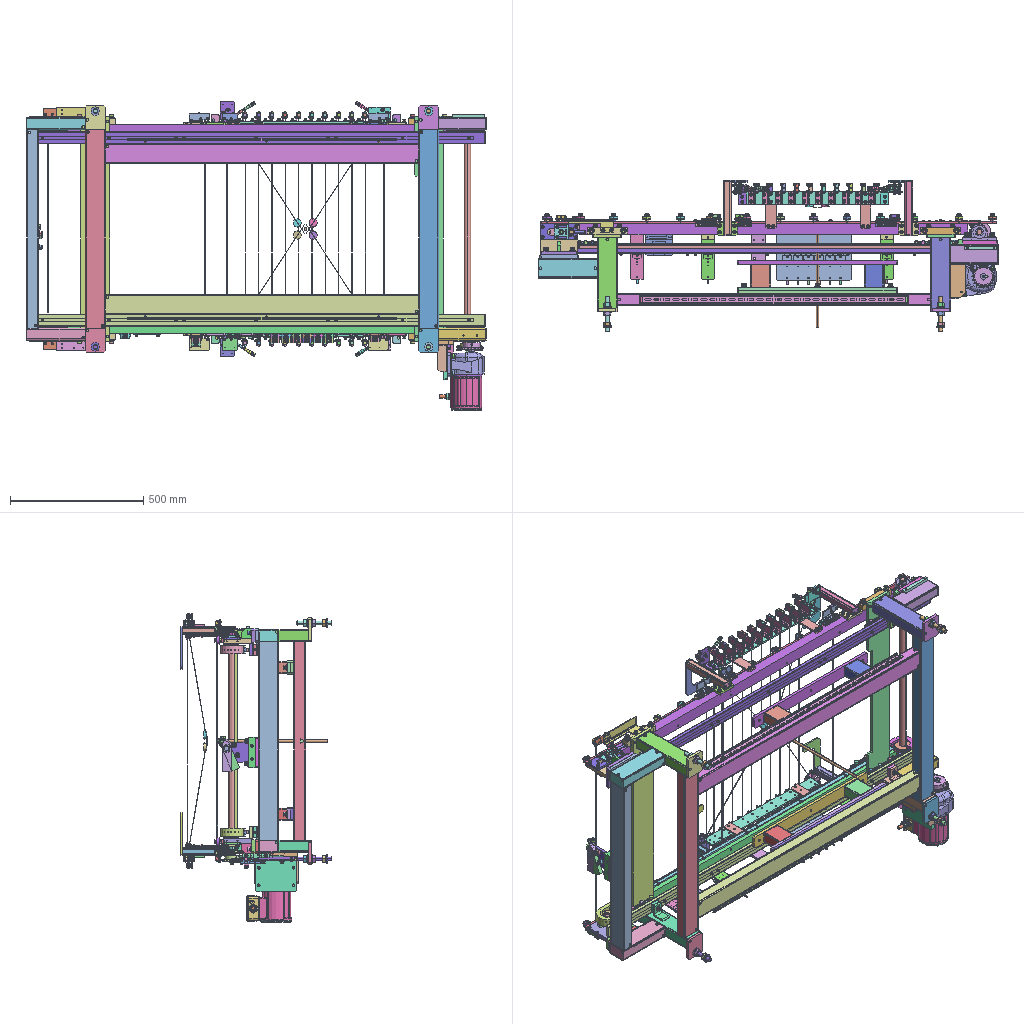Assembly | STEP file | 1685 different items | 2041 placed | box 1725 x 566 x 1158 mm
Parts list (item | name | quantity | parent item | size | volume), first 292 of 1685 items:
1 | 30B-162015T | x1 | in J306-EBZ05-01-40 | 15 x 20 x 20 mm | 1686 mm3
2 | AJSTS8-45 | x1 | in [1 unit purchased part] | 78 x 15.011 x 13 mm | 5597 mm3
3 | BB62-M10-25L | x1 | in J013-EBZ05-13-06 | 16 x 35 x 16 mm | 3564 mm3
4 | BB62-M10-25L-1 | x1 | in J013-EBZ05-13-06 | 16 x 35 x 16 mm | 3564 mm3
5 | BB62-M10-25L-10 | x1 | in J013-EBZ05-13-06 | 16 x 35 x 16 mm | 3564 mm3
6 | BB62-M10-25L-11 | x1 | in J013-EBZ05-13-06 | 16 x 35 x 16 mm | 3564 mm3
7 | BB62-M10-25L-12 | x1 | in J013-EBZ05-13-06 | 16 x 35 x 16 mm | 3564 mm3
8 | BB62-M10-25L-13 | x1 | in J013-EBZ05-13-06 | 16 x 35 x 16 mm | 3564 mm3
9 | BB62-M10-25L-14 | x1 | in J013-EBZ05-12-06 | 16 x 35 x 16 mm | 3564 mm3
10 | BB62-M10-25L-15 | x1 | in J013-EBZ05-12-06 | 16 x 35 x 16 mm | 3564 mm3
11 | BB62-M10-25L-16 | x1 | in J013-EBZ05-12-06 | 16 x 35 x 16 mm | 3564 mm3
12 | BB62-M10-25L-17 | x1 | in J013-EBZ05-12-06 | 16 x 35 x 16 mm | 3564 mm3
13 | BB62-M10-25L-18 | x1 | in J013-EBZ05-12-06 | 16 x 35 x 16 mm | 3564 mm3
14 | BB62-M10-25L-19 | x1 | in J013-EBZ05-12-06 | 16 x 35 x 16 mm | 3564 mm3
15 | BB62-M10-25L-2 | x1 | in J013-EBZ05-13-06 | 16 x 35 x 16 mm | 3564 mm3
16 | BB62-M10-25L-20 | x1 | in J013-EBZ05-12-06 | 16 x 35 x 16 mm | 3564 mm3
17 | BB62-M10-25L-21 | x1 | in J013-EBZ05-12-06 | 16 x 35 x 16 mm | 3564 mm3
18 | BB62-M10-25L-22 | x1 | in J013-EBZ05-12-06 | 16 x 35 x 16 mm | 3564 mm3
19 | BB62-M10-25L-23 | x1 | in J013-EBZ05-12-06 | 16 x 35 x 16 mm | 3564 mm3
20 | BB62-M10-25L-24 | x1 | in J013-EBZ05-12-06 | 16 x 35 x 16 mm | 3564 mm3
21 | BB62-M10-25L-25 | x1 | in J013-EBZ05-12-06 | 16 x 35 x 16 mm | 3564 mm3
22 | BB62-M10-25L-26 | x1 | in J013-EBZ05-12-06 | 16 x 35 x 16 mm | 3564 mm3
23 | BB62-M10-25L-27 | x1 | in J013-EBZ05-12-06 | 16 x 35 x 16 mm | 3564 mm3
24 | BB62-M10-25L-3 | x1 | in J013-EBZ05-13-06 | 16 x 35 x 16 mm | 3564 mm3
25 | BB62-M10-25L-4 | x1 | in J013-EBZ05-13-06 | 16 x 35 x 16 mm | 3564 mm3
26 | BB62-M10-25L-5 | x1 | in J013-EBZ05-13-06 | 16 x 35 x 16 mm | 3564 mm3
27 | BB62-M10-25L-6 | x1 | in J013-EBZ05-13-06 | 16 x 35 x 16 mm | 3564 mm3
28 | BB62-M10-25L-7 | x1 | in J013-EBZ05-13-06 | 16 x 35 x 16 mm | 3564 mm3
29 | BB62-M10-25L-8 | x1 | in J013-EBZ05-13-06 | 16 x 35 x 16 mm | 3564 mm3
30 | BB62-M10-25L-9 | x1 | in J013-EBZ05-13-06 | 16 x 35 x 16 mm | 3564 mm3
31 | BB62-M10-30L | x1 | in [1 unit purchased part] | 16 x 40 x 16 mm | 3957 mm3
32 | BB62-M10-30L-1 | x1 | in [1 unit purchased part] | 16 x 40 x 16 mm | 3957 mm3
33 | BB62-M10-30L-10 | x1 | - | 16 x 40 x 16 mm | 3957 mm3
34 | BB62-M10-30L-11 | x1 | - | 16 x 40 x 16 mm | 3957 mm3
35 | BB62-M10-30L-2 | x1 | in [1 unit purchased part] | 16 x 40 x 16 mm | 3957 mm3
36 | BB62-M10-30L-3 | x1 | in [1 unit purchased part] | 16 x 40 x 16 mm | 3957 mm3
37 | BB62-M10-30L-4 | x1 | - | 16 x 40 x 16 mm | 3957 mm3
38 | BB62-M10-30L-5 | x1 | - | 16 x 40 x 16 mm | 3957 mm3
39 | BB62-M10-30L-6 | x1 | - | 16 x 40 x 16 mm | 3957 mm3
40 | BB62-M10-30L-7 | x1 | - | 16 x 40 x 16 mm | 3957 mm3
41 | BB62-M10-30L-8 | x1 | - | 16 x 40 x 16 mm | 3957 mm3
42 | BB62-M10-30L-9 | x1 | - | 16 x 40 x 16 mm | 3957 mm3
43 | BB62-M10-35L | x1 | - | 16 x 45 x 16 mm | 4350 mm3
44 | BB62-M10-35L-1 | x1 | - | 16 x 45 x 16 mm | 4350 mm3
45 | BB62-M10-35L-2 | x1 | - | 16 x 45 x 16 mm | 4350 mm3
46 | BB62-M10-35L-3 | x1 | - | 16 x 45 x 16 mm | 4350 mm3
47 | BB62-M10-40L | x2 | in J013-EBZ05-14-06 | 16 x 50 x 16 mm | 4742 mm3
48 | BB62-M10-40L-1 | x2 | in J013-EBZ05-14-06 | 16 x 50 x 16 mm | 4742 mm3
49 | BB62-M10-40L-2 | x2 | in J013-EBZ05-28-06 | 16 x 50 x 16 mm | 4742 mm3
50 | BB62-M10-40L-3 | x2 | in J013-EBZ05-28-06 | 16 x 50 x 16 mm | 4742 mm3
51 | BB62-M10-40L-4 | x1 | - | 16 x 50 x 16 mm | 4742 mm3
52 | BB62-M10-40L-5 | x1 | - | 16 x 50 x 16 mm | 4742 mm3
53 | BB62-M10-45L | x2 | in J013-EBZ05-14-06 | 16 x 55 x 16 mm | 5135 mm3
54 | BB62-M10-45L-1 | x2 | in J013-EBZ05-14-06 | 16 x 55 x 16 mm | 5135 mm3
55 | BB62-M10-45L-2 | x2 | in J013-EBZ05-28-06 | 16 x 55 x 16 mm | 5135 mm3
56 | BB62-M10-45L-3 | x2 | in J013-EBZ05-28-06 | 16 x 55 x 16 mm | 5135 mm3
57 | BB62-M12-30L | x2 | in J011-EBZ05-05-00 | 18 x 42 x 18 mm | 5695 mm3
58 | BB62-M12-30L-1 | x2 | in J011-EBZ05-05-00 | 18 x 42 x 18 mm | 5695 mm3
59 | BB62-M3-10L | x1 | - | 5.5 x 13 x 5.5 mm | 130.673 mm3
60 | BB62-M3-10L-1 | x1 | - | 5.5 x 13 x 5.5 mm | 130.673 mm3
61 | BB62-M3-10L-10 | x10 | in J014-EBZ05-07-06 | 5.5 x 13 x 5.5 mm | 130.673 mm3
62 | BB62-M3-10L-11 | x10 | in J014-EBZ05-07-06 | 5.5 x 13 x 5.5 mm | 130.673 mm3
63 | BB62-M3-10L-12 | x1 | in J014-EBZ05-13-06 | 5.5 x 13 x 5.5 mm | 130.673 mm3
64 | BB62-M3-10L-13 | x1 | in J014-EBZ05-13-06 | 5.5 x 13 x 5.5 mm | 130.673 mm3
65 | BB62-M3-10L-14 | x1 | in J014-EBZ05-14-06 | 5.5 x 13 x 5.5 mm | 130.673 mm3
66 | BB62-M3-10L-15 | x1 | in J014-EBZ05-14-06 | 5.5 x 13 x 5.5 mm | 130.673 mm3
67 | BB62-M3-10L-16 | x1 | - | 5.5 x 13 x 5.5 mm | 130.673 mm3
68 | BB62-M3-10L-17 | x1 | - | 5.5 x 13 x 5.5 mm | 130.673 mm3
69 | BB62-M3-10L-18 | x1 | - | 5.5 x 13 x 5.5 mm | 130.673 mm3
70 | BB62-M3-10L-19 | x1 | - | 5.5 x 13 x 5.5 mm | 130.673 mm3
71 | BB62-M3-10L-2 | x1 | - | 5.5 x 13 x 5.5 mm | 130.673 mm3
72 | BB62-M3-10L-20 | x1 | - | 5.5 x 13 x 5.5 mm | 130.673 mm3
73 | BB62-M3-10L-21 | x1 | - | 5.5 x 13 x 5.5 mm | 130.673 mm3
74 | BB62-M3-10L-22 | x1 | - | 5.5 x 13 x 5.5 mm | 130.673 mm3
75 | BB62-M3-10L-23 | x1 | - | 5.5 x 13 x 5.5 mm | 130.673 mm3
76 | BB62-M3-10L-3 | x1 | - | 5.5 x 13 x 5.5 mm | 130.673 mm3
77 | BB62-M3-10L-4 | x2 | in J014-EBZ05-02-06 | 5.5 x 13 x 5.5 mm | 130.673 mm3
78 | BB62-M3-10L-5 | x2 | in J014-EBZ05-02-06 | 5.5 x 13 x 5.5 mm | 130.673 mm3
79 | BB62-M3-10L-6 | x2 | in J014-EBZ05-01-06 | 5.5 x 13 x 5.5 mm | 130.673 mm3
80 | BB62-M3-10L-7 | x2 | in J014-EBZ05-01-06 | 5.5 x 13 x 5.5 mm | 130.673 mm3
81 | BB62-M3-10L-8 | x10 | in J014-EBZ05-06-06 | 5.5 x 13 x 5.5 mm | 130.673 mm3
82 | BB62-M3-10L-9 | x10 | in J014-EBZ05-06-06 | 5.5 x 13 x 5.5 mm | 130.673 mm3
83 | BB62-M4-15L | x1 | in J013-EBZ05-05-06 | 7 x 19 x 7 mm | 317.881 mm3
84 | BB62-M4-15L-1 | x1 | in J013-EBZ05-05-06 | 7 x 19 x 7 mm | 317.881 mm3
85 | BB62-M4-15L-10 | x1 | in J013-EBZ05-06-06 | 7 x 19 x 7 mm | 317.881 mm3
86 | BB62-M4-15L-11 | x1 | in J013-EBZ05-06-06 | 7 x 19 x 7 mm | 317.881 mm3
87 | BB62-M4-15L-12 | x1 | in J013-EBZ05-06-06 | 7 x 19 x 7 mm | 317.881 mm3
88 | BB62-M4-15L-13 | x1 | in J013-EBZ05-06-06 | 7 x 19 x 7 mm | 317.881 mm3
89 | BB62-M4-15L-14 | x1 | in J013-EBZ05-06-06 | 7 x 19 x 7 mm | 317.881 mm3
90 | BB62-M4-15L-15 | x1 | in J013-EBZ05-06-06 | 7 x 19 x 7 mm | 317.881 mm3
91 | BB62-M4-15L-2 | x1 | in J013-EBZ05-05-06 | 7 x 19 x 7 mm | 317.881 mm3
92 | BB62-M4-15L-3 | x1 | in J013-EBZ05-05-06 | 7 x 19 x 7 mm | 317.881 mm3
93 | BB62-M4-15L-4 | x1 | in J013-EBZ05-05-06 | 7 x 19 x 7 mm | 317.881 mm3
94 | BB62-M4-15L-5 | x1 | in J013-EBZ05-05-06 | 7 x 19 x 7 mm | 317.881 mm3
95 | BB62-M4-15L-6 | x1 | in J013-EBZ05-05-06 | 7 x 19 x 7 mm | 317.881 mm3
96 | BB62-M4-15L-7 | x1 | in J013-EBZ05-05-06 | 7 x 19 x 7 mm | 317.881 mm3
97 | BB62-M4-15L-8 | x1 | in J013-EBZ05-06-06 | 7 x 19 x 7 mm | 317.881 mm3
98 | BB62-M4-15L-9 | x1 | in J013-EBZ05-06-06 | 7 x 19 x 7 mm | 317.881 mm3
99 | BB62-M4-20L | x1 | - | 7 x 24 x 7 mm | 380.713 mm3
100 | BB62-M4-20L-1 | x1 | - | 7 x 24 x 7 mm | 380.713 mm3
101 | BB62-M4-20L-2 | x1 | - | 7 x 24 x 7 mm | 380.713 mm3
102 | BB62-M4-20L-3 | x1 | - | 7 x 24 x 7 mm | 380.713 mm3
103 | BB62-M4-20L-4 | x1 | - | 7 x 24 x 7 mm | 380.713 mm3
104 | BB62-M4-20L-5 | x1 | - | 7 x 24 x 7 mm | 380.713 mm3
105 | BB62-M4-35L | x1 | - | 7 x 39 x 7 mm | 569.208 mm3
106 | BB62-M4-35L-1 | x1 | - | 7 x 39 x 7 mm | 569.208 mm3
107 | BB62-M4-35L-10 | x1 | - | 7 x 39 x 7 mm | 569.208 mm3
108 | BB62-M4-35L-11 | x1 | - | 7 x 39 x 7 mm | 569.208 mm3
109 | BB62-M4-35L-12 | x1 | - | 7 x 39 x 7 mm | 569.208 mm3
110 | BB62-M4-35L-13 | x1 | - | 7 x 39 x 7 mm | 569.208 mm3
111 | BB62-M4-35L-14 | x1 | - | 7 x 39 x 7 mm | 569.208 mm3
112 | BB62-M4-35L-15 | x1 | - | 7 x 39 x 7 mm | 569.208 mm3
113 | BB62-M4-35L-16 | x1 | - | 7 x 39 x 7 mm | 569.208 mm3
114 | BB62-M4-35L-17 | x1 | - | 7 x 39 x 7 mm | 569.208 mm3
115 | BB62-M4-35L-2 | x1 | - | 7 x 39 x 7 mm | 569.208 mm3
116 | BB62-M4-35L-3 | x1 | - | 7 x 39 x 7 mm | 569.208 mm3
117 | BB62-M4-35L-4 | x1 | - | 7 x 39 x 7 mm | 569.208 mm3
118 | BB62-M4-35L-5 | x1 | - | 7 x 39 x 7 mm | 569.208 mm3
119 | BB62-M4-35L-6 | x1 | - | 7 x 39 x 7 mm | 569.208 mm3
120 | BB62-M4-35L-7 | x1 | - | 7 x 39 x 7 mm | 569.208 mm3
121 | BB62-M4-35L-8 | x1 | - | 7 x 39 x 7 mm | 569.208 mm3
122 | BB62-M4-35L-9 | x1 | - | 7 x 39 x 7 mm | 569.208 mm3
123 | BB62-M5-10L | x2 | in J014-EBZ05-03-06 | 8.5 x 15 x 8.5 mm | 427.848 mm3
124 | BB62-M5-10L-1 | x2 | in J014-EBZ05-03-06 | 8.5 x 15 x 8.5 mm | 427.848 mm3
125 | BB62-M5-10L-2 | x1 | in J014-EBZ05-18-06 | 8.5 x 15 x 8.5 mm | 427.848 mm3
126 | BB62-M5-10L-3 | x1 | in J014-EBZ05-18-06 | 8.5 x 15 x 8.5 mm | 427.848 mm3
127 | BB62-M5-12L | x1 | - | 8.5 x 17 x 8.5 mm | 467.118 mm3
128 | BB62-M5-12L-1 | x1 | - | 8.5 x 17 x 8.5 mm | 467.118 mm3
129 | BB62-M5-12L-10 | x1 | - | 8.5 x 17 x 8.5 mm | 467.118 mm3
130 | BB62-M5-12L-11 | x1 | - | 8.5 x 17 x 8.5 mm | 467.118 mm3
131 | BB62-M5-12L-12 | x10 | in J014-EBZ05-06-06 | 8.5 x 17 x 8.5 mm | 467.118 mm3
132 | BB62-M5-12L-13 | x10 | in J014-EBZ05-06-06 | 8.5 x 17 x 8.5 mm | 467.118 mm3
133 | BB62-M5-12L-14 | x10 | in J014-EBZ05-07-06 | 8.5 x 17 x 8.5 mm | 467.118 mm3
134 | BB62-M5-12L-15 | x10 | in J014-EBZ05-07-06 | 8.5 x 17 x 8.5 mm | 467.118 mm3
135 | BB62-M5-12L-16 | x1 | in J014-EBZ05-13-06 | 8.5 x 17 x 8.5 mm | 467.118 mm3
136 | BB62-M5-12L-17 | x1 | in J014-EBZ05-13-06 | 8.5 x 17 x 8.5 mm | 467.118 mm3
137 | BB62-M5-12L-18 | x1 | in J014-EBZ05-14-06 | 8.5 x 17 x 8.5 mm | 467.118 mm3
138 | BB62-M5-12L-19 | x1 | in J014-EBZ05-14-06 | 8.5 x 17 x 8.5 mm | 467.118 mm3
139 | BB62-M5-12L-2 | x1 | - | 8.5 x 17 x 8.5 mm | 467.118 mm3
140 | BB62-M5-12L-20 | x1 | in J014-EBZ05-09-06 | 8.5 x 17 x 8.5 mm | 467.118 mm3
141 | BB62-M5-12L-21 | x1 | in J014-EBZ05-09-06 | 8.5 x 17 x 8.5 mm | 467.118 mm3
142 | BB62-M5-12L-22 | x1 | - | 8.5 x 17 x 8.5 mm | 467.118 mm3
143 | BB62-M5-12L-23 | x1 | - | 8.5 x 17 x 8.5 mm | 467.118 mm3
144 | BB62-M5-12L-24 | x1 | - | 8.5 x 17 x 8.5 mm | 467.118 mm3
145 | BB62-M5-12L-25 | x1 | - | 8.5 x 17 x 8.5 mm | 467.118 mm3
146 | BB62-M5-12L-26 | x1 | - | 8.5 x 17 x 8.5 mm | 467.118 mm3
147 | BB62-M5-12L-27 | x1 | - | 8.5 x 17 x 8.5 mm | 467.118 mm3
148 | BB62-M5-12L-28 | x1 | - | 8.5 x 17 x 8.5 mm | 467.118 mm3
149 | BB62-M5-12L-29 | x1 | - | 8.5 x 17 x 8.5 mm | 467.118 mm3
150 | BB62-M5-12L-3 | x1 | - | 8.5 x 17 x 8.5 mm | 467.118 mm3
151 | BB62-M5-12L-30 | x1 | in J014-EBZ05-08-06 | 8.5 x 17 x 8.5 mm | 467.118 mm3
152 | BB62-M5-12L-31 | x1 | in J014-EBZ05-08-06 | 8.5 x 17 x 8.5 mm | 467.118 mm3
153 | BB62-M5-12L-32 | x1 | in J014-EBZ05-10-06 | 8.5 x 17 x 8.5 mm | 467.118 mm3
154 | BB62-M5-12L-33 | x1 | in J014-EBZ05-10-06 | 8.5 x 17 x 8.5 mm | 467.118 mm3
155 | BB62-M5-12L-34 | x1 | in J014-EBZ05-11-06 | 8.5 x 17 x 8.5 mm | 467.118 mm3
156 | BB62-M5-12L-35 | x1 | in J014-EBZ05-11-06 | 8.5 x 17 x 8.5 mm | 467.118 mm3
157 | BB62-M5-12L-4 | x1 | - | 8.5 x 17 x 8.5 mm | 467.118 mm3
158 | BB62-M5-12L-5 | x1 | - | 8.5 x 17 x 8.5 mm | 467.118 mm3
159 | BB62-M5-12L-6 | x1 | - | 8.5 x 17 x 8.5 mm | 467.118 mm3
160 | BB62-M5-12L-7 | x1 | - | 8.5 x 17 x 8.5 mm | 467.118 mm3
161 | BB62-M5-12L-8 | x1 | - | 8.5 x 17 x 8.5 mm | 467.118 mm3
162 | BB62-M5-12L-9 | x1 | - | 8.5 x 17 x 8.5 mm | 467.118 mm3
163 | BB62-M5-15L | x1 | - | 8.5 x 20 x 8.5 mm | 526.023 mm3
164 | BB62-M5-15L-1 | x1 | - | 8.5 x 20 x 8.5 mm | 526.023 mm3
165 | BB62-M5-15L-2 | x1 | - | 8.5 x 20 x 8.5 mm | 526.023 mm3
166 | BB62-M5-15L-3 | x1 | - | 8.5 x 20 x 8.5 mm | 526.023 mm3
167 | BB62-M5-15L-4 | x1 | - | 8.5 x 20 x 8.5 mm | 526.023 mm3
168 | BB62-M5-15L-5 | x1 | - | 8.5 x 20 x 8.5 mm | 526.023 mm3
169 | BB62-M5-15L-6 | x1 | - | 8.5 x 20 x 8.5 mm | 526.023 mm3
170 | BB62-M5-15L-7 | x1 | - | 8.5 x 20 x 8.5 mm | 526.023 mm3
171 | BB62-M5-20L | x1 | in J013-EBZ05-13-06 | 8.5 x 25 x 8.5 mm | 624.198 mm3
172 | BB62-M5-20L-1 | x1 | in J013-EBZ05-13-06 | 8.5 x 25 x 8.5 mm | 624.198 mm3
173 | BB62-M5-20L-2 | x1 | in J013-EBZ05-13-06 | 8.5 x 25 x 8.5 mm | 624.198 mm3
174 | BB62-M5-20L-3 | x1 | in J013-EBZ05-13-06 | 8.5 x 25 x 8.5 mm | 624.198 mm3
175 | BB62-M5-20L-4 | x1 | in J013-EBZ05-12-06 | 8.5 x 25 x 8.5 mm | 624.198 mm3
176 | BB62-M5-20L-5 | x1 | in J013-EBZ05-12-06 | 8.5 x 25 x 8.5 mm | 624.198 mm3
177 | BB62-M5-20L-6 | x1 | in J013-EBZ05-12-06 | 8.5 x 25 x 8.5 mm | 624.198 mm3
178 | BB62-M5-20L-7 | x1 | in J013-EBZ05-12-06 | 8.5 x 25 x 8.5 mm | 624.198 mm3
179 | BB62-M5-25L | x2 | in J013-EBZ05-27-06 | 8.5 x 30 x 8.5 mm | 722.372 mm3
180 | BB62-M5-25L-1 | x2 | in J013-EBZ05-27-06 | 8.5 x 30 x 8.5 mm | 722.372 mm3
181 | BB62-M6-12L | x1 | in J014-EBZ05-15-06 | 10 x 18 x 10 mm | 713.399 mm3
182 | BB62-M6-12L-1 | x1 | in J014-EBZ05-15-06 | 10 x 18 x 10 mm | 713.399 mm3
183 | BB62-M6-12L-2 | x1 | in J014-EBZ05-16-06 | 10 x 18 x 10 mm | 713.399 mm3
184 | BB62-M6-12L-3 | x1 | in J014-EBZ05-16-06 | 10 x 18 x 10 mm | 713.399 mm3
185 | BB62-M6-15L | x1 | in J013-EBZ05-15-06 | 10 x 21 x 10 mm | 798.222 mm3
186 | BB62-M6-15L-1 | x1 | in J013-EBZ05-15-06 | 10 x 21 x 10 mm | 798.222 mm3
187 | BB62-M6-15L-10 | x1 | in J014-EBZ05-12-06 | 10 x 21 x 10 mm | 798.222 mm3
188 | BB62-M6-15L-11 | x1 | in J014-EBZ05-12-06 | 10 x 21 x 10 mm | 798.222 mm3
189 | BB62-M6-15L-2 | x1 | - | 10 x 21 x 10 mm | 798.222 mm3
190 | BB62-M6-15L-3 | x1 | - | 10 x 21 x 10 mm | 798.222 mm3
191 | BB62-M6-15L-4 | x1 | - | 10 x 21 x 10 mm | 798.222 mm3
192 | BB62-M6-15L-5 | x1 | - | 10 x 21 x 10 mm | 798.222 mm3
193 | BB62-M6-15L-6 | x1 | - | 10 x 21 x 10 mm | 798.222 mm3
194 | BB62-M6-15L-7 | x1 | - | 10 x 21 x 10 mm | 798.222 mm3
195 | BB62-M6-15L-8 | x1 | - | 10 x 21 x 10 mm | 798.222 mm3
196 | BB62-M6-15L-9 | x1 | - | 10 x 21 x 10 mm | 798.222 mm3
197 | BB62-M6-18L | x1 | in J013-EBZ05-05-06 | 10 x 24 x 10 mm | 883.045 mm3
198 | BB62-M6-18L-1 | x1 | in J013-EBZ05-05-06 | 10 x 24 x 10 mm | 883.045 mm3
199 | BB62-M6-18L-10 | x1 | in J013-EBZ05-06-06 | 10 x 24 x 10 mm | 883.045 mm3
200 | BB62-M6-18L-11 | x1 | in J013-EBZ05-06-06 | 10 x 24 x 10 mm | 883.045 mm3
201 | BB62-M6-18L-2 | x1 | in J013-EBZ05-05-06 | 10 x 24 x 10 mm | 883.045 mm3
202 | BB62-M6-18L-3 | x1 | in J013-EBZ05-05-06 | 10 x 24 x 10 mm | 883.045 mm3
203 | BB62-M6-18L-4 | x1 | in J013-EBZ05-05-06 | 10 x 24 x 10 mm | 883.045 mm3
204 | BB62-M6-18L-5 | x1 | in J013-EBZ05-05-06 | 10 x 24 x 10 mm | 883.045 mm3
205 | BB62-M6-18L-6 | x1 | in J013-EBZ05-06-06 | 10 x 24 x 10 mm | 883.045 mm3
206 | BB62-M6-18L-7 | x1 | in J013-EBZ05-06-06 | 10 x 24 x 10 mm | 883.045 mm3
207 | BB62-M6-18L-8 | x1 | in J013-EBZ05-06-06 | 10 x 24 x 10 mm | 883.045 mm3
208 | BB62-M6-18L-9 | x1 | in J013-EBZ05-06-06 | 10 x 24 x 10 mm | 883.045 mm3
209 | BB62-M6-20L | x1 | - | 10 x 26 x 10 mm | 939.593 mm3
210 | BB62-M6-20L-1 | x1 | - | 10 x 26 x 10 mm | 939.593 mm3
211 | BB62-M6-20L-10 | x1 | - | 10 x 26 x 10 mm | 939.593 mm3
212 | BB62-M6-20L-11 | x1 | - | 10 x 26 x 10 mm | 939.593 mm3
213 | BB62-M6-20L-12 | x1 | - | 10 x 26 x 10 mm | 939.593 mm3
214 | BB62-M6-20L-13 | x1 | - | 10 x 26 x 10 mm | 939.593 mm3
215 | BB62-M6-20L-14 | x1 | - | 10 x 26 x 10 mm | 939.593 mm3
216 | BB62-M6-20L-15 | x1 | - | 10 x 26 x 10 mm | 939.593 mm3
217 | BB62-M6-20L-16 | x1 | - | 10 x 26 x 10 mm | 939.593 mm3
218 | BB62-M6-20L-17 | x1 | - | 10 x 26 x 10 mm | 939.593 mm3
219 | BB62-M6-20L-18 | x1 | - | 10 x 26 x 10 mm | 939.593 mm3
220 | BB62-M6-20L-19 | x1 | - | 10 x 26 x 10 mm | 939.593 mm3
221 | BB62-M6-20L-2 | x1 | - | 10 x 26 x 10 mm | 939.593 mm3
222 | BB62-M6-20L-20 | x1 | - | 10 x 26 x 10 mm | 939.593 mm3
223 | BB62-M6-20L-21 | x1 | - | 10 x 26 x 10 mm | 939.593 mm3
224 | BB62-M6-20L-22 | x1 | - | 10 x 26 x 10 mm | 939.593 mm3
225 | BB62-M6-20L-23 | x1 | - | 10 x 26 x 10 mm | 939.593 mm3
226 | BB62-M6-20L-24 | x1 | - | 10 x 26 x 10 mm | 939.593 mm3
227 | BB62-M6-20L-25 | x1 | - | 10 x 26 x 10 mm | 939.593 mm3
228 | BB62-M6-20L-3 | x1 | - | 10 x 26 x 10 mm | 939.593 mm3
229 | BB62-M6-20L-4 | x1 | - | 10 x 26 x 10 mm | 939.593 mm3
230 | BB62-M6-20L-5 | x1 | - | 10 x 26 x 10 mm | 939.593 mm3
231 | BB62-M6-20L-6 | x1 | - | 10 x 26 x 10 mm | 939.593 mm3
232 | BB62-M6-20L-7 | x1 | - | 10 x 26 x 10 mm | 939.593 mm3
233 | BB62-M6-20L-8 | x4 | in J014-EBZ05-04-06 | 10 x 26 x 10 mm | 939.593 mm3
234 | BB62-M6-20L-9 | x4 | in J014-EBZ05-04-06 | 10 x 26 x 10 mm | 939.593 mm3
235 | BB62-M8-15L | x1 | in [1 unit purchased part] | 13 x 23 x 13 mm | 1627 mm3
236 | BB62-M8-15L-1 | x1 | in J013-EBZ05-26-06 | 13 x 23 x 13 mm | 1627 mm3
237 | BB62-M8-15L-2 | x1 | in J013-EBZ05-26-06 | 13 x 23 x 13 mm | 1627 mm3
238 | BB62-M8-20L | x1 | - | 13 x 28 x 13 mm | 1878 mm3
239 | BB62-M8-20L-1 | x1 | - | 13 x 28 x 13 mm | 1878 mm3
240 | BB62-M8-20L-2 | x1 | - | 13 x 28 x 13 mm | 1878 mm3
241 | BB62-M8-20L-3 | x1 | - | 13 x 28 x 13 mm | 1878 mm3
242 | BB62-M8-25L | x1 | in J015-EBZ05-06-06 | 13 x 33 x 13 mm | 2129 mm3
243 | BB62-M8-25L-1 | x1 | in J015-EBZ05-06-06 | 13 x 33 x 13 mm | 2129 mm3
244 | BB62-M8-30L | x1 | in J011-EBZ05-01-06 | 13 x 38 x 13 mm | 2381 mm3
245 | BB62-M8-30L-1 | x1 | in J011-EBZ05-01-06 | 13 x 38 x 13 mm | 2381 mm3
246 | BB62-M8-30L-2 | x1 | in J011-EBZ05-01-06 | 13 x 38 x 13 mm | 2381 mm3
247 | BB62-M8-30L-3 | x1 | in J011-EBZ05-01-06 | 13 x 38 x 13 mm | 2381 mm3
248 | BB62-M8-50L | x1 | in J011-EBZ05-02-00 | 13 x 58 x 13 mm | 3386 mm3
249 | BB62-M8-50L-1 | x1 | in J011-EBZ05-02-00 | 13 x 58 x 13 mm | 3386 mm3
250 | BB67-M16-130L | x1 | - | 130 x 16 x 16 mm | 26090 mm3
251 | BB67-M16-130L-1 | x1 | - | 130 x 16 x 16 mm | 26090 mm3
252 | BB67-M16-130L-2 | x1 | - | 130 x 16 x 16 mm | 26090 mm3
253 | BB67-M16-130L-3 | x1 | - | 130 x 16 x 16 mm | 26090 mm3
254 | C-SB6200ZZ | x1 | in J013-EBZ05-13-06 | 9 x 30 x 30 mm | 5496 mm3
255 | C-SB6200ZZ-1 | x1 | in J013-EBZ05-13-06 | 9 x 30 x 30 mm | 5496 mm3
256 | C-SB6200ZZ-10 | x1 | in J013-EBZ05-13-06 | 9 x 30 x 30 mm | 5496 mm3
257 | C-SB6200ZZ-11 | x1 | in J013-EBZ05-13-06 | 9 x 30 x 30 mm | 5496 mm3
258 | C-SB6200ZZ-12 | x1 | in J013-EBZ05-13-06 | 9 x 30 x 30 mm | 5496 mm3
259 | C-SB6200ZZ-13 | x1 | in J013-EBZ05-13-06 | 9 x 30 x 30 mm | 5496 mm3
260 | C-SB6200ZZ-14 | x1 | in J013-EBZ05-12-06 | 9 x 30 x 30 mm | 5496 mm3
261 | C-SB6200ZZ-15 | x1 | in J013-EBZ05-12-06 | 9 x 30 x 30 mm | 5496 mm3
262 | C-SB6200ZZ-16 | x1 | in J013-EBZ05-12-06 | 9 x 30 x 30 mm | 5496 mm3
263 | C-SB6200ZZ-17 | x1 | in J013-EBZ05-12-06 | 9 x 30 x 30 mm | 5496 mm3
264 | C-SB6200ZZ-18 | x1 | in J013-EBZ05-12-06 | 9 x 30 x 30 mm | 5496 mm3
265 | C-SB6200ZZ-19 | x1 | in J013-EBZ05-12-06 | 9 x 30 x 30 mm | 5496 mm3
266 | C-SB6200ZZ-2 | x1 | in J013-EBZ05-13-06 | 9 x 30 x 30 mm | 5496 mm3
267 | C-SB6200ZZ-20 | x1 | in J013-EBZ05-12-06 | 9 x 30 x 30 mm | 5496 mm3
268 | C-SB6200ZZ-21 | x1 | in J013-EBZ05-12-06 | 9 x 30 x 30 mm | 5496 mm3
269 | C-SB6200ZZ-22 | x1 | in J013-EBZ05-12-06 | 9 x 30 x 30 mm | 5496 mm3
270 | C-SB6200ZZ-23 | x1 | in J013-EBZ05-12-06 | 9 x 30 x 30 mm | 5496 mm3
271 | C-SB6200ZZ-24 | x1 | in J013-EBZ05-12-06 | 9 x 30 x 30 mm | 5496 mm3
272 | C-SB6200ZZ-25 | x1 | in J013-EBZ05-12-06 | 9 x 30 x 30 mm | 5496 mm3
273 | C-SB6200ZZ-26 | x1 | in J013-EBZ05-12-06 | 9 x 30 x 30 mm | 5496 mm3
274 | C-SB6200ZZ-27 | x1 | in J013-EBZ05-12-06 | 9 x 30 x 30 mm | 5496 mm3
275 | C-SB6200ZZ-3 | x1 | in J013-EBZ05-13-06 | 9 x 30 x 30 mm | 5496 mm3
276 | C-SB6200ZZ-4 | x1 | in J013-EBZ05-13-06 | 9 x 30 x 30 mm | 5496 mm3
277 | C-SB6200ZZ-5 | x1 | in J013-EBZ05-13-06 | 9 x 30 x 30 mm | 5496 mm3
278 | C-SB6200ZZ-6 | x1 | in J013-EBZ05-13-06 | 9 x 30 x 30 mm | 5496 mm3
279 | C-SB6200ZZ-7 | x1 | in J013-EBZ05-13-06 | 9 x 30 x 30 mm | 5496 mm3
280 | C-SB6200ZZ-8 | x1 | in J013-EBZ05-13-06 | 9 x 30 x 30 mm | 5496 mm3
281 | C-SB6200ZZ-9 | x1 | in J013-EBZ05-13-06 | 9 x 30 x 30 mm | 5496 mm3
282 | CBSST5-12 | x1 | - | 15.5 x 8.5 x 8.5 mm | 408.692 mm3
283 | CBSST5-12-1 | x1 | - | 15.5 x 8.5 x 8.5 mm | 408.692 mm3
284 | CBSST5-12-10 | x1 | - | 15.5 x 8.5 x 8.5 mm | 408.692 mm3
285 | CBSST5-12-11 | x1 | - | 15.5 x 8.5 x 8.5 mm | 408.692 mm3
286 | CBSST5-12-2 | x1 | - | 15.5 x 8.5 x 8.5 mm | 408.692 mm3
287 | CBSST5-12-3 | x1 | - | 15.5 x 8.5 x 8.5 mm | 408.692 mm3
288 | CBSST5-12-4 | x1 | - | 15.5 x 8.5 x 8.5 mm | 408.692 mm3
289 | CBSST5-12-5 | x1 | - | 15.5 x 8.5 x 8.5 mm | 408.692 mm3
290 | CBSST5-12-6 | x1 | - | 15.5 x 8.5 x 8.5 mm | 408.692 mm3
291 | CBSST5-12-7 | x1 | - | 15.5 x 8.5 x 8.5 mm | 408.692 mm3
292 | CBSST5-12-8 | x1 | - | 15.5 x 8.5 x 8.5 mm | 408.692 mm3